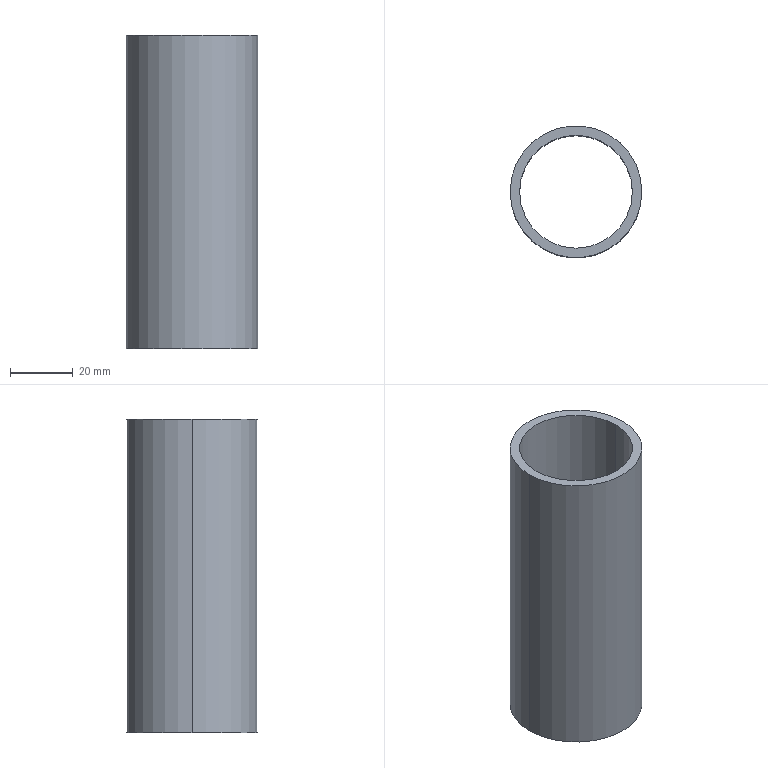Part | SolidWorks | features Extrusion 1 | 1 solid | 6 faces | box 42 x 42 x 100 mm | volume 36757 mm3 | cylinder 4 | plane 2 | commonest cylinder face diameters 36 x2 42 x2
STEP:
#1=CARTESIAN_POINT('',(-18.,0.,100.));
#2=VERTEX_POINT('',#1);
#3=CARTESIAN_POINT('',(18.,0.,100.));
#4=VERTEX_POINT('',#3);
#5=CARTESIAN_POINT('',(0.,0.,100.));
#6=DIRECTION('',(0.,0.,1.));
#7=DIRECTION('',(1.,0.,0.));
#8=AXIS2_PLACEMENT_3D('',#5,#6,#7);
#9=CIRCLE('',#8,18.);
#10=EDGE_CURVE('',#2,#4,#9,.T.);
#11=ORIENTED_EDGE('',*,*,#10,.T.);
#12=CARTESIAN_POINT('',(18.,0.,0.));
#13=VERTEX_POINT('',#12);
#14=CARTESIAN_POINT('',(18.,0.,100.));
#15=DIRECTION('',(0.,0.,-1.));
#16=VECTOR('',#15,1000.);
#17=LINE('',#14,#16);
#18=EDGE_CURVE('',#4,#13,#17,.T.);
#19=ORIENTED_EDGE('',*,*,#18,.T.);
#20=CARTESIAN_POINT('',(-18.,0.,0.));
#21=VERTEX_POINT('',#20);
#22=CARTESIAN_POINT('',(0.,0.,0.));
#23=DIRECTION('',(0.,0.,1.));
#24=DIRECTION('',(1.,0.,0.));
#25=AXIS2_PLACEMENT_3D('',#22,#23,#24);
#26=CIRCLE('',#25,18.);
#27=EDGE_CURVE('',#21,#13,#26,.T.);
#28=ORIENTED_EDGE('',*,*,#27,.F.);
#29=CARTESIAN_POINT('',(-18.,0.,100.));
#30=DIRECTION('',(0.,0.,-1.));
#31=VECTOR('',#30,1000.);
#32=LINE('',#29,#31);
#33=EDGE_CURVE('',#2,#21,#32,.T.);
#34=ORIENTED_EDGE('',*,*,#33,.F.);
#35=EDGE_LOOP('',(#11,#19,#28,#34));
#36=FACE_OUTER_BOUND('',#35,.T.);
#37=CARTESIAN_POINT('',(0.,0.,100.));
#38=DIRECTION('',(0.,0.,-1.));
#39=DIRECTION('',(-1.,0.,0.));
#40=AXIS2_PLACEMENT_3D('',#37,#38,#39);
#41=CYLINDRICAL_SURFACE('',#40,18.);
#42=ADVANCED_FACE('',(#36),#41,.F.);
#43=CARTESIAN_POINT('',(21.,0.,100.));
#44=VERTEX_POINT('',#43);
#45=CARTESIAN_POINT('',(-21.,0.,100.));
#46=VERTEX_POINT('',#45);
#47=CARTESIAN_POINT('',(0.,0.,100.));
#48=DIRECTION('',(0.,0.,1.));
#49=DIRECTION('',(1.,0.,0.));
#50=AXIS2_PLACEMENT_3D('',#47,#48,#49);
#51=CIRCLE('',#50,21.);
#52=EDGE_CURVE('',#44,#46,#51,.T.);
#53=ORIENTED_EDGE('',*,*,#52,.F.);
#54=CARTESIAN_POINT('',(21.,0.,0.));
#55=VERTEX_POINT('',#54);
#56=CARTESIAN_POINT('',(21.,0.,100.));
#57=DIRECTION('',(0.,0.,-1.));
#58=VECTOR('',#57,1000.);
#59=LINE('',#56,#58);
#60=EDGE_CURVE('',#44,#55,#59,.T.);
#61=ORIENTED_EDGE('',*,*,#60,.T.);
#62=CARTESIAN_POINT('',(-21.,0.,0.));
#63=VERTEX_POINT('',#62);
#64=CARTESIAN_POINT('',(0.,0.,0.));
#65=DIRECTION('',(0.,0.,1.));
#66=DIRECTION('',(1.,0.,0.));
#67=AXIS2_PLACEMENT_3D('',#64,#65,#66);
#68=CIRCLE('',#67,21.);
#69=EDGE_CURVE('',#55,#63,#68,.T.);
#70=ORIENTED_EDGE('',*,*,#69,.T.);
#71=CARTESIAN_POINT('',(-21.,0.,100.));
#72=DIRECTION('',(0.,0.,-1.));
#73=VECTOR('',#72,1000.);
#74=LINE('',#71,#73);
#75=EDGE_CURVE('',#46,#63,#74,.T.);
#76=ORIENTED_EDGE('',*,*,#75,.F.);
#77=EDGE_LOOP('',(#53,#61,#70,#76));
#78=FACE_OUTER_BOUND('',#77,.T.);
#79=CARTESIAN_POINT('',(0.,0.,100.));
#80=DIRECTION('',(0.,0.,-1.));
#81=DIRECTION('',(-1.,0.,0.));
#82=AXIS2_PLACEMENT_3D('',#79,#80,#81);
#83=CYLINDRICAL_SURFACE('',#82,21.);
#84=ADVANCED_FACE('',(#78),#83,.T.);
#85=CARTESIAN_POINT('',(0.,0.,100.));
#86=DIRECTION('',(0.,0.,1.));
#87=DIRECTION('',(1.,0.,0.));
#88=AXIS2_PLACEMENT_3D('',#85,#86,#87);
#89=CIRCLE('',#88,21.);
#90=EDGE_CURVE('',#46,#44,#89,.T.);
#91=ORIENTED_EDGE('',*,*,#90,.T.);
#92=ORIENTED_EDGE('',*,*,#52,.T.);
#93=EDGE_LOOP('',(#91,#92));
#94=FACE_OUTER_BOUND('',#93,.T.);
#95=ORIENTED_EDGE('',*,*,#10,.F.);
#96=CARTESIAN_POINT('',(0.,0.,100.));
#97=DIRECTION('',(0.,0.,1.));
#98=DIRECTION('',(1.,0.,0.));
#99=AXIS2_PLACEMENT_3D('',#96,#97,#98);
#100=CIRCLE('',#99,18.);
#101=EDGE_CURVE('',#4,#2,#100,.T.);
#102=ORIENTED_EDGE('',*,*,#101,.F.);
#103=EDGE_LOOP('',(#95,#102));
#104=FACE_BOUND('',#103,.T.);
#105=CARTESIAN_POINT('',(0.,0.,100.));
#106=DIRECTION('',(0.,0.,1.));
#107=DIRECTION('',(1.,0.,0.));
#108=AXIS2_PLACEMENT_3D('',#105,#106,#107);
#109=PLANE('',#108);
#110=ADVANCED_FACE('',(#94,#104),#109,.T.);
#111=CARTESIAN_POINT('',(0.,0.,0.));
#112=DIRECTION('',(0.,0.,1.));
#113=DIRECTION('',(1.,0.,0.));
#114=AXIS2_PLACEMENT_3D('',#111,#112,#113);
#115=CIRCLE('',#114,21.);
#116=EDGE_CURVE('',#63,#55,#115,.T.);
#117=ORIENTED_EDGE('',*,*,#116,.F.);
#118=ORIENTED_EDGE('',*,*,#69,.F.);
#119=EDGE_LOOP('',(#117,#118));
#120=FACE_OUTER_BOUND('',#119,.T.);
#121=ORIENTED_EDGE('',*,*,#27,.T.);
#122=CARTESIAN_POINT('',(0.,0.,0.));
#123=DIRECTION('',(0.,0.,1.));
#124=DIRECTION('',(1.,0.,0.));
#125=AXIS2_PLACEMENT_3D('',#122,#123,#124);
#126=CIRCLE('',#125,18.);
#127=EDGE_CURVE('',#13,#21,#126,.T.);
#128=ORIENTED_EDGE('',*,*,#127,.T.);
#129=EDGE_LOOP('',(#121,#128));
#130=FACE_BOUND('',#129,.T.);
#131=CARTESIAN_POINT('',(0.,0.,0.));
#132=DIRECTION('',(0.,0.,1.));
#133=DIRECTION('',(1.,0.,0.));
#134=AXIS2_PLACEMENT_3D('',#131,#132,#133);
#135=PLANE('',#134);
#136=ADVANCED_FACE('',(#120,#130),#135,.F.);
#137=ORIENTED_EDGE('',*,*,#60,.F.);
#138=ORIENTED_EDGE('',*,*,#90,.F.);
#139=ORIENTED_EDGE('',*,*,#75,.T.);
#140=ORIENTED_EDGE('',*,*,#116,.T.);
#141=EDGE_LOOP('',(#137,#138,#139,#140));
#142=FACE_OUTER_BOUND('',#141,.T.);
#143=CARTESIAN_POINT('',(0.,0.,100.));
#144=DIRECTION('',(0.,0.,-1.));
#145=DIRECTION('',(-1.,0.,0.));
#146=AXIS2_PLACEMENT_3D('',#143,#144,#145);
#147=CYLINDRICAL_SURFACE('',#146,21.);
#148=ADVANCED_FACE('',(#142),#147,.T.);
#149=ORIENTED_EDGE('',*,*,#18,.F.);
#150=ORIENTED_EDGE('',*,*,#101,.T.);
#151=ORIENTED_EDGE('',*,*,#33,.T.);
#152=ORIENTED_EDGE('',*,*,#127,.F.);
#153=EDGE_LOOP('',(#149,#150,#151,#152));
#154=FACE_OUTER_BOUND('',#153,.T.);
#155=CARTESIAN_POINT('',(0.,0.,100.));
#156=DIRECTION('',(0.,0.,-1.));
#157=DIRECTION('',(-1.,0.,0.));
#158=AXIS2_PLACEMENT_3D('',#155,#156,#157);
#159=CYLINDRICAL_SURFACE('',#158,18.);
#160=ADVANCED_FACE('',(#154),#159,.F.);
#161=CLOSED_SHELL('',(#42,#84,#110,#136,#148,#160));
#162=MANIFOLD_SOLID_BREP('',#161);
#163=CARTESIAN_POINT('',(0.,0.,0.));
#164=DIRECTION('',(0.,0.,1.));
#165=DIRECTION('',(1.,0.,0.));
#166=AXIS2_PLACEMENT_3D('',#163,#164,#165);
#167=(LENGTH_UNIT()NAMED_UNIT(*)SI_UNIT(.MILLI.,.METRE.));
#168=UNCERTAINTY_MEASURE_WITH_UNIT(LENGTH_MEASURE(0.00001),#167,'','');
#169=(NAMED_UNIT(*)PLANE_ANGLE_UNIT()SI_UNIT($,.RADIAN.));
#170=(NAMED_UNIT(*)SI_UNIT($,.STERADIAN.)SOLID_ANGLE_UNIT());
#171=(GEOMETRIC_REPRESENTATION_CONTEXT(3)GLOBAL_UNCERTAINTY_ASSIGNED_CONTEXT((#168))GLOBAL_UNIT_ASSIGNED_CONTEXT((#167,#169,#170))REPRESENTATION_CONTEXT('',''));
#172=ADVANCED_BREP_SHAPE_REPRESENTATION('',(#162,#166),#171);